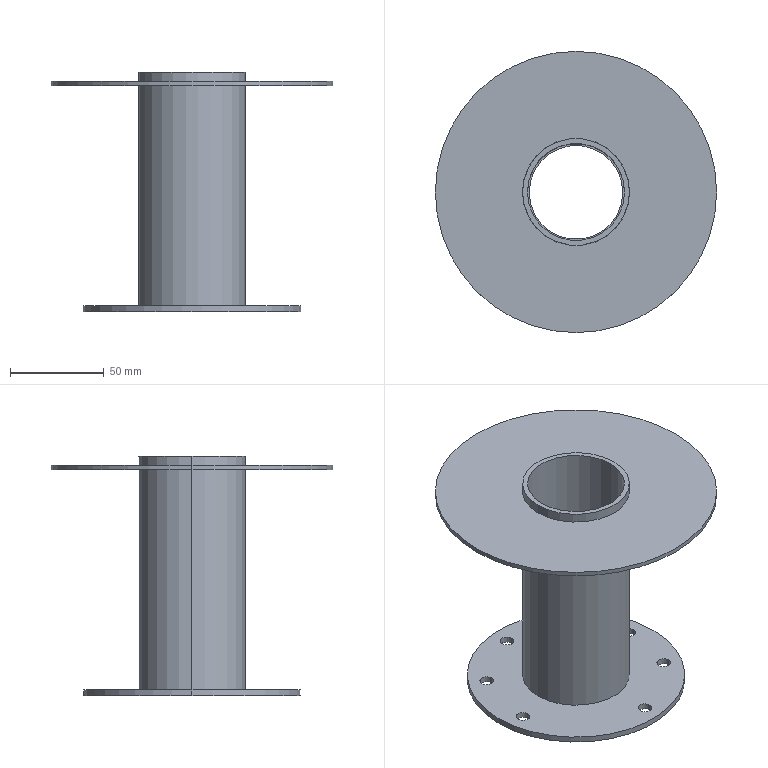Part | SolidWorks | features BaseBody 5 | 3 solids | 30 faces | box 150 x 150 x 127.9 mm | volume 116898 mm3 | cylinder 24 | plane 6 | commonest cylinder face diameters 7.2 x12 50 x2 51.8 x2 57 x2 57.2 x2 116 x2
STEP:
#1=CARTESIAN_POINT('',(-38.144,24.146,84.393));
#2=VERTEX_POINT('',#1);
#3=CARTESIAN_POINT('',(19.056,24.146,84.393));
#4=VERTEX_POINT('',#3);
#5=CARTESIAN_POINT('',(-9.544,24.146,84.393));
#6=DIRECTION('',(0.,0.,1.));
#7=DIRECTION('',(1.,0.,0.));
#8=AXIS2_PLACEMENT_3D('',#5,#6,#7);
#9=CIRCLE('',#8,28.6);
#10=EDGE_CURVE('',#2,#4,#9,.T.);
#11=ORIENTED_EDGE('',*,*,#10,.F.);
#12=CARTESIAN_POINT('',(-38.144,24.146,86.693));
#13=VERTEX_POINT('',#12);
#14=CARTESIAN_POINT('',(-38.144,24.146,84.393));
#15=DIRECTION('',(0.,0.,1.));
#16=VECTOR('',#15,1000.);
#17=LINE('',#14,#16);
#18=EDGE_CURVE('',#2,#13,#17,.T.);
#19=ORIENTED_EDGE('',*,*,#18,.T.);
#20=CARTESIAN_POINT('',(19.056,24.146,86.693));
#21=VERTEX_POINT('',#20);
#22=CARTESIAN_POINT('',(-9.544,24.146,86.693));
#23=DIRECTION('',(0.,0.,1.));
#24=DIRECTION('',(1.,0.,0.));
#25=AXIS2_PLACEMENT_3D('',#22,#23,#24);
#26=CIRCLE('',#25,28.6);
#27=EDGE_CURVE('',#13,#21,#26,.T.);
#28=ORIENTED_EDGE('',*,*,#27,.T.);
#29=CARTESIAN_POINT('',(19.056,24.146,84.393));
#30=DIRECTION('',(0.,0.,1.));
#31=VECTOR('',#30,1000.);
#32=LINE('',#29,#31);
#33=EDGE_CURVE('',#4,#21,#32,.T.);
#34=ORIENTED_EDGE('',*,*,#33,.F.);
#35=EDGE_LOOP('',(#11,#19,#28,#34));
#36=FACE_OUTER_BOUND('',#35,.T.);
#37=CARTESIAN_POINT('',(-9.544,24.146,84.393));
#38=DIRECTION('',(0.,0.,1.));
#39=DIRECTION('',(1.,0.,0.));
#40=AXIS2_PLACEMENT_3D('',#37,#38,#39);
#41=CYLINDRICAL_SURFACE('',#40,28.6);
#42=ADVANCED_FACE('',(#36),#41,.F.);
#43=CARTESIAN_POINT('',(65.456,24.146,84.393));
#44=VERTEX_POINT('',#43);
#45=CARTESIAN_POINT('',(-84.544,24.146,84.393));
#46=VERTEX_POINT('',#45);
#47=CARTESIAN_POINT('',(-9.544,24.146,84.393));
#48=DIRECTION('',(0.,0.,1.));
#49=DIRECTION('',(1.,0.,0.));
#50=AXIS2_PLACEMENT_3D('',#47,#48,#49);
#51=CIRCLE('',#50,75.);
#52=EDGE_CURVE('',#44,#46,#51,.T.);
#53=ORIENTED_EDGE('',*,*,#52,.T.);
#54=CARTESIAN_POINT('',(-84.544,24.146,86.693));
#55=VERTEX_POINT('',#54);
#56=CARTESIAN_POINT('',(-84.544,24.146,84.393));
#57=DIRECTION('',(0.,0.,1.));
#58=VECTOR('',#57,1000.);
#59=LINE('',#56,#58);
#60=EDGE_CURVE('',#46,#55,#59,.T.);
#61=ORIENTED_EDGE('',*,*,#60,.T.);
#62=CARTESIAN_POINT('',(65.456,24.146,86.693));
#63=VERTEX_POINT('',#62);
#64=CARTESIAN_POINT('',(-9.544,24.146,86.693));
#65=DIRECTION('',(0.,0.,1.));
#66=DIRECTION('',(1.,0.,0.));
#67=AXIS2_PLACEMENT_3D('',#64,#65,#66);
#68=CIRCLE('',#67,75.);
#69=EDGE_CURVE('',#63,#55,#68,.T.);
#70=ORIENTED_EDGE('',*,*,#69,.F.);
#71=CARTESIAN_POINT('',(65.456,24.146,84.393));
#72=DIRECTION('',(0.,0.,1.));
#73=VECTOR('',#72,1000.);
#74=LINE('',#71,#73);
#75=EDGE_CURVE('',#44,#63,#74,.T.);
#76=ORIENTED_EDGE('',*,*,#75,.F.);
#77=EDGE_LOOP('',(#53,#61,#70,#76));
#78=FACE_OUTER_BOUND('',#77,.T.);
#79=CARTESIAN_POINT('',(-9.544,24.146,84.393));
#80=DIRECTION('',(0.,0.,1.));
#81=DIRECTION('',(1.,0.,0.));
#82=AXIS2_PLACEMENT_3D('',#79,#80,#81);
#83=CYLINDRICAL_SURFACE('',#82,75.);
#84=ADVANCED_FACE('',(#78),#83,.T.);
#85=ORIENTED_EDGE('',*,*,#60,.F.);
#86=CARTESIAN_POINT('',(-9.544,24.146,84.393));
#87=DIRECTION('',(0.,0.,1.));
#88=DIRECTION('',(1.,0.,0.));
#89=AXIS2_PLACEMENT_3D('',#86,#87,#88);
#90=CIRCLE('',#89,75.);
#91=EDGE_CURVE('',#46,#44,#90,.T.);
#92=ORIENTED_EDGE('',*,*,#91,.T.);
#93=ORIENTED_EDGE('',*,*,#75,.T.);
#94=CARTESIAN_POINT('',(-9.544,24.146,86.693));
#95=DIRECTION('',(0.,0.,1.));
#96=DIRECTION('',(1.,0.,0.));
#97=AXIS2_PLACEMENT_3D('',#94,#95,#96);
#98=CIRCLE('',#97,75.);
#99=EDGE_CURVE('',#55,#63,#98,.T.);
#100=ORIENTED_EDGE('',*,*,#99,.F.);
#101=EDGE_LOOP('',(#85,#92,#93,#100));
#102=FACE_OUTER_BOUND('',#101,.T.);
#103=CARTESIAN_POINT('',(-9.544,24.146,84.393));
#104=DIRECTION('',(0.,0.,1.));
#105=DIRECTION('',(1.,0.,0.));
#106=AXIS2_PLACEMENT_3D('',#103,#104,#105);
#107=CYLINDRICAL_SURFACE('',#106,75.);
#108=ADVANCED_FACE('',(#102),#107,.T.);
#109=CARTESIAN_POINT('',(-9.544,24.146,84.393));
#110=DIRECTION('',(0.,0.,1.));
#111=DIRECTION('',(1.,0.,0.));
#112=AXIS2_PLACEMENT_3D('',#109,#110,#111);
#113=CIRCLE('',#112,28.6);
#114=EDGE_CURVE('',#4,#2,#113,.T.);
#115=ORIENTED_EDGE('',*,*,#114,.T.);
#116=ORIENTED_EDGE('',*,*,#10,.T.);
#117=EDGE_LOOP('',(#115,#116));
#118=FACE_BOUND('',#117,.T.);
#119=ORIENTED_EDGE('',*,*,#52,.F.);
#120=ORIENTED_EDGE('',*,*,#91,.F.);
#121=EDGE_LOOP('',(#119,#120));
#122=FACE_OUTER_BOUND('',#121,.T.);
#123=CARTESIAN_POINT('',(-9.544,24.146,84.393));
#124=DIRECTION('',(0.,0.,1.));
#125=DIRECTION('',(1.,0.,0.));
#126=AXIS2_PLACEMENT_3D('',#123,#124,#125);
#127=PLANE('',#126);
#128=ADVANCED_FACE('',(#118,#122),#127,.F.);
#129=CARTESIAN_POINT('',(-9.544,24.146,86.693));
#130=DIRECTION('',(0.,0.,1.));
#131=DIRECTION('',(1.,0.,0.));
#132=AXIS2_PLACEMENT_3D('',#129,#130,#131);
#133=CIRCLE('',#132,28.6);
#134=EDGE_CURVE('',#21,#13,#133,.T.);
#135=ORIENTED_EDGE('',*,*,#134,.F.);
#136=ORIENTED_EDGE('',*,*,#27,.F.);
#137=EDGE_LOOP('',(#135,#136));
#138=FACE_BOUND('',#137,.T.);
#139=ORIENTED_EDGE('',*,*,#69,.T.);
#140=ORIENTED_EDGE('',*,*,#99,.T.);
#141=EDGE_LOOP('',(#139,#140));
#142=FACE_OUTER_BOUND('',#141,.T.);
#143=CARTESIAN_POINT('',(-9.544,24.146,86.693));
#144=DIRECTION('',(0.,0.,1.));
#145=DIRECTION('',(1.,0.,0.));
#146=AXIS2_PLACEMENT_3D('',#143,#144,#145);
#147=PLANE('',#146);
#148=ADVANCED_FACE('',(#138,#142),#147,.T.);
#149=ORIENTED_EDGE('',*,*,#18,.F.);
#150=ORIENTED_EDGE('',*,*,#114,.F.);
#151=ORIENTED_EDGE('',*,*,#33,.T.);
#152=ORIENTED_EDGE('',*,*,#134,.T.);
#153=EDGE_LOOP('',(#149,#150,#151,#152));
#154=FACE_OUTER_BOUND('',#153,.T.);
#155=CARTESIAN_POINT('',(-9.544,24.146,84.393));
#156=DIRECTION('',(0.,0.,1.));
#157=DIRECTION('',(1.,0.,0.));
#158=AXIS2_PLACEMENT_3D('',#155,#156,#157);
#159=CYLINDRICAL_SURFACE('',#158,28.6);
#160=ADVANCED_FACE('',(#154),#159,.F.);
#161=CLOSED_SHELL('',(#42,#84,#108,#128,#148,#160));
#162=MANIFOLD_SOLID_BREP('',#161);
#163=CARTESIAN_POINT('',(-35.444,24.146,91.693));
#164=VERTEX_POINT('',#163);
#165=CARTESIAN_POINT('',(16.356,24.146,91.693));
#166=VERTEX_POINT('',#165);
#167=CARTESIAN_POINT('',(-9.544,24.146,91.693));
#168=DIRECTION('',(0.,0.,1.));
#169=DIRECTION('',(1.,0.,0.));
#170=AXIS2_PLACEMENT_3D('',#167,#168,#169);
#171=CIRCLE('',#170,25.9);
#172=EDGE_CURVE('',#164,#166,#171,.T.);
#173=ORIENTED_EDGE('',*,*,#172,.T.);
#174=CARTESIAN_POINT('',(16.356,24.146,-33.007));
#175=VERTEX_POINT('',#174);
#176=CARTESIAN_POINT('',(16.356,24.146,91.693));
#177=DIRECTION('',(0.,0.,-1.));
#178=VECTOR('',#177,1000.);
#179=LINE('',#176,#178);
#180=EDGE_CURVE('',#166,#175,#179,.T.);
#181=ORIENTED_EDGE('',*,*,#180,.T.);
#182=CARTESIAN_POINT('',(-35.444,24.146,-33.007));
#183=VERTEX_POINT('',#182);
#184=CARTESIAN_POINT('',(-9.544,24.146,-33.007));
#185=DIRECTION('',(0.,0.,1.));
#186=DIRECTION('',(1.,0.,0.));
#187=AXIS2_PLACEMENT_3D('',#184,#185,#186);
#188=CIRCLE('',#187,25.9);
#189=EDGE_CURVE('',#183,#175,#188,.T.);
#190=ORIENTED_EDGE('',*,*,#189,.F.);
#191=CARTESIAN_POINT('',(-35.444,24.146,91.693));
#192=DIRECTION('',(0.,0.,-1.));
#193=VECTOR('',#192,1000.);
#194=LINE('',#191,#193);
#195=EDGE_CURVE('',#164,#183,#194,.T.);
#196=ORIENTED_EDGE('',*,*,#195,.F.);
#197=EDGE_LOOP('',(#173,#181,#190,#196));
#198=FACE_OUTER_BOUND('',#197,.T.);
#199=CARTESIAN_POINT('',(-9.544,24.146,91.693));
#200=DIRECTION('',(0.,0.,-1.));
#201=DIRECTION('',(-1.,0.,0.));
#202=AXIS2_PLACEMENT_3D('',#199,#200,#201);
#203=CYLINDRICAL_SURFACE('',#202,25.9);
#204=ADVANCED_FACE('',(#198),#203,.F.);
#205=CARTESIAN_POINT('',(18.956,24.146,91.693));
#206=VERTEX_POINT('',#205);
#207=CARTESIAN_POINT('',(-38.044,24.146,91.693));
#208=VERTEX_POINT('',#207);
#209=CARTESIAN_POINT('',(-9.544,24.146,91.693));
#210=DIRECTION('',(0.,0.,1.));
#211=DIRECTION('',(1.,0.,0.));
#212=AXIS2_PLACEMENT_3D('',#209,#210,#211);
#213=CIRCLE('',#212,28.5);
#214=EDGE_CURVE('',#206,#208,#213,.T.);
#215=ORIENTED_EDGE('',*,*,#214,.F.);
#216=CARTESIAN_POINT('',(18.956,24.146,-33.007));
#217=VERTEX_POINT('',#216);
#218=CARTESIAN_POINT('',(18.956,24.146,91.693));
#219=DIRECTION('',(0.,0.,-1.));
#220=VECTOR('',#219,1000.);
#221=LINE('',#218,#220);
#222=EDGE_CURVE('',#206,#217,#221,.T.);
#223=ORIENTED_EDGE('',*,*,#222,.T.);
#224=CARTESIAN_POINT('',(-38.044,24.146,-33.007));
#225=VERTEX_POINT('',#224);
#226=CARTESIAN_POINT('',(-9.544,24.146,-33.007));
#227=DIRECTION('',(0.,0.,1.));
#228=DIRECTION('',(1.,0.,0.));
#229=AXIS2_PLACEMENT_3D('',#226,#227,#228);
#230=CIRCLE('',#229,28.5);
#231=EDGE_CURVE('',#217,#225,#230,.T.);
#232=ORIENTED_EDGE('',*,*,#231,.T.);
#233=CARTESIAN_POINT('',(-38.044,24.146,91.693));
#234=DIRECTION('',(0.,0.,-1.));
#235=VECTOR('',#234,1000.);
#236=LINE('',#233,#235);
#237=EDGE_CURVE('',#208,#225,#236,.T.);
#238=ORIENTED_EDGE('',*,*,#237,.F.);
#239=EDGE_LOOP('',(#215,#223,#232,#238));
#240=FACE_OUTER_BOUND('',#239,.T.);
#241=CARTESIAN_POINT('',(-9.544,24.146,91.693));
#242=DIRECTION('',(0.,0.,-1.));
#243=DIRECTION('',(-1.,0.,0.));
#244=AXIS2_PLACEMENT_3D('',#241,#242,#243);
#245=CYLINDRICAL_SURFACE('',#244,28.5);
#246=ADVANCED_FACE('',(#240),#245,.T.);
#247=CARTESIAN_POINT('',(-9.544,24.146,91.693));
#248=DIRECTION('',(0.,0.,1.));
#249=DIRECTION('',(1.,0.,0.));
#250=AXIS2_PLACEMENT_3D('',#247,#248,#249);
#251=CIRCLE('',#250,28.5);
#252=EDGE_CURVE('',#208,#206,#251,.T.);
#253=ORIENTED_EDGE('',*,*,#252,.T.);
#254=ORIENTED_EDGE('',*,*,#214,.T.);
#255=EDGE_LOOP('',(#253,#254));
#256=FACE_OUTER_BOUND('',#255,.T.);
#257=ORIENTED_EDGE('',*,*,#172,.F.);
#258=CARTESIAN_POINT('',(-9.544,24.146,91.693));
#259=DIRECTION('',(0.,0.,1.));
#260=DIRECTION('',(1.,0.,0.));
#261=AXIS2_PLACEMENT_3D('',#258,#259,#260);
#262=CIRCLE('',#261,25.9);
#263=EDGE_CURVE('',#166,#164,#262,.T.);
#264=ORIENTED_EDGE('',*,*,#263,.F.);
#265=EDGE_LOOP('',(#257,#264));
#266=FACE_BOUND('',#265,.T.);
#267=CARTESIAN_POINT('',(-9.544,24.146,91.693));
#268=DIRECTION('',(0.,0.,1.));
#269=DIRECTION('',(1.,0.,0.));
#270=AXIS2_PLACEMENT_3D('',#267,#268,#269);
#271=PLANE('',#270);
#272=ADVANCED_FACE('',(#256,#266),#271,.T.);
#273=CARTESIAN_POINT('',(-9.544,24.146,-33.007));
#274=DIRECTION('',(0.,0.,1.));
#275=DIRECTION('',(1.,0.,0.));
#276=AXIS2_PLACEMENT_3D('',#273,#274,#275);
#277=CIRCLE('',#276,28.5);
#278=EDGE_CURVE('',#225,#217,#277,.T.);
#279=ORIENTED_EDGE('',*,*,#278,.F.);
#280=ORIENTED_EDGE('',*,*,#231,.F.);
#281=EDGE_LOOP('',(#279,#280));
#282=FACE_OUTER_BOUND('',#281,.T.);
#283=ORIENTED_EDGE('',*,*,#189,.T.);
#284=CARTESIAN_POINT('',(-9.544,24.146,-33.007));
#285=DIRECTION('',(0.,0.,1.));
#286=DIRECTION('',(1.,0.,0.));
#287=AXIS2_PLACEMENT_3D('',#284,#285,#286);
#288=CIRCLE('',#287,25.9);
#289=EDGE_CURVE('',#175,#183,#288,.T.);
#290=ORIENTED_EDGE('',*,*,#289,.T.);
#291=EDGE_LOOP('',(#283,#290));
#292=FACE_BOUND('',#291,.T.);
#293=CARTESIAN_POINT('',(-9.544,24.146,-33.007));
#294=DIRECTION('',(0.,0.,1.));
#295=DIRECTION('',(1.,0.,0.));
#296=AXIS2_PLACEMENT_3D('',#293,#294,#295);
#297=PLANE('',#296);
#298=ADVANCED_FACE('',(#282,#292),#297,.F.);
#299=ORIENTED_EDGE('',*,*,#222,.F.);
#300=ORIENTED_EDGE('',*,*,#252,.F.);
#301=ORIENTED_EDGE('',*,*,#237,.T.);
#302=ORIENTED_EDGE('',*,*,#278,.T.);
#303=EDGE_LOOP('',(#299,#300,#301,#302));
#304=FACE_OUTER_BOUND('',#303,.T.);
#305=CARTESIAN_POINT('',(-9.544,24.146,91.693));
#306=DIRECTION('',(0.,0.,-1.));
#307=DIRECTION('',(-1.,0.,0.));
#308=AXIS2_PLACEMENT_3D('',#305,#306,#307);
#309=CYLINDRICAL_SURFACE('',#308,28.5);
#310=ADVANCED_FACE('',(#304),#309,.T.);
#311=ORIENTED_EDGE('',*,*,#180,.F.);
#312=ORIENTED_EDGE('',*,*,#263,.T.);
#313=ORIENTED_EDGE('',*,*,#195,.T.);
#314=ORIENTED_EDGE('',*,*,#289,.F.);
#315=EDGE_LOOP('',(#311,#312,#313,#314));
#316=FACE_OUTER_BOUND('',#315,.T.);
#317=CARTESIAN_POINT('',(-9.544,24.146,91.693));
#318=DIRECTION('',(0.,0.,-1.));
#319=DIRECTION('',(-1.,0.,0.));
#320=AXIS2_PLACEMENT_3D('',#317,#318,#319);
#321=CYLINDRICAL_SURFACE('',#320,25.9);
#322=ADVANCED_FACE('',(#316),#321,.F.);
#323=CLOSED_SHELL('',(#204,#246,#272,#298,#310,#322));
#324=MANIFOLD_SOLID_BREP('',#323);
#325=CARTESIAN_POINT('',(-17.328,71.964,-33.007));
#326=VERTEX_POINT('',#325);
#327=CARTESIAN_POINT('',(-10.128,71.964,-33.007));
#328=VERTEX_POINT('',#327);
#329=CARTESIAN_POINT('',(-13.728,71.964,-33.007));
#330=DIRECTION('',(0.,0.,-1.));
#331=DIRECTION('',(1.,0.,0.));
#332=AXIS2_PLACEMENT_3D('',#329,#330,#331);
#333=CIRCLE('',#332,3.6);
#334=EDGE_CURVE('',#326,#328,#333,.T.);
#335=ORIENTED_EDGE('',*,*,#334,.F.);
#336=CARTESIAN_POINT('',(-17.328,71.964,-36.207));
#337=VERTEX_POINT('',#336);
#338=CARTESIAN_POINT('',(-17.328,71.964,-33.007));
#339=DIRECTION('',(0.,0.,-1.));
#340=VECTOR('',#339,1000.);
#341=LINE('',#338,#340);
#342=EDGE_CURVE('',#326,#337,#341,.T.);
#343=ORIENTED_EDGE('',*,*,#342,.T.);
#344=CARTESIAN_POINT('',(-10.128,71.964,-36.207));
#345=VERTEX_POINT('',#344);
#346=CARTESIAN_POINT('',(-13.728,71.964,-36.207));
#347=DIRECTION('',(0.,0.,-1.));
#348=DIRECTION('',(1.,0.,0.));
#349=AXIS2_PLACEMENT_3D('',#346,#347,#348);
#350=CIRCLE('',#349,3.6);
#351=EDGE_CURVE('',#337,#345,#350,.T.);
#352=ORIENTED_EDGE('',*,*,#351,.T.);
#353=CARTESIAN_POINT('',(-10.128,71.964,-33.007));
#354=DIRECTION('',(0.,0.,-1.));
#355=VECTOR('',#354,1000.);
#356=LINE('',#353,#355);
#357=EDGE_CURVE('',#328,#345,#356,.T.);
#358=ORIENTED_EDGE('',*,*,#357,.F.);
#359=EDGE_LOOP('',(#335,#343,#352,#358));
#360=FACE_OUTER_BOUND('',#359,.T.);
#361=CARTESIAN_POINT('',(-13.728,71.964,-33.007));
#362=DIRECTION('',(0.,0.,-1.));
#363=DIRECTION('',(1.,0.,0.));
#364=AXIS2_PLACEMENT_3D('',#361,#362,#363);
#365=CYLINDRICAL_SURFACE('',#364,3.6);
#366=ADVANCED_FACE('',(#360),#365,.F.);
#367=CARTESIAN_POINT('',(-50.969,53.698,-33.007));
#368=VERTEX_POINT('',#367);
#369=CARTESIAN_POINT('',(-43.769,53.698,-33.007));
#370=VERTEX_POINT('',#369);
#371=CARTESIAN_POINT('',(-47.369,53.698,-33.007));
#372=DIRECTION('',(0.,0.,-1.));
#373=DIRECTION('',(1.,0.,0.));
#374=AXIS2_PLACEMENT_3D('',#371,#372,#373);
#375=CIRCLE('',#374,3.6);
#376=EDGE_CURVE('',#368,#370,#375,.T.);
#377=ORIENTED_EDGE('',*,*,#376,.F.);
#378=CARTESIAN_POINT('',(-50.969,53.698,-36.207));
#379=VERTEX_POINT('',#378);
#380=CARTESIAN_POINT('',(-50.969,53.698,-33.007));
#381=DIRECTION('',(0.,0.,-1.));
#382=VECTOR('',#381,1000.);
#383=LINE('',#380,#382);
#384=EDGE_CURVE('',#368,#379,#383,.T.);
#385=ORIENTED_EDGE('',*,*,#384,.T.);
#386=CARTESIAN_POINT('',(-43.769,53.698,-36.207));
#387=VERTEX_POINT('',#386);
#388=CARTESIAN_POINT('',(-47.369,53.698,-36.207));
#389=DIRECTION('',(0.,0.,-1.));
#390=DIRECTION('',(1.,0.,0.));
#391=AXIS2_PLACEMENT_3D('',#388,#389,#390);
#392=CIRCLE('',#391,3.6);
#393=EDGE_CURVE('',#379,#387,#392,.T.);
#394=ORIENTED_EDGE('',*,*,#393,.T.);
#395=CARTESIAN_POINT('',(-43.769,53.698,-33.007));
#396=DIRECTION('',(0.,0.,-1.));
#397=VECTOR('',#396,1000.);
#398=LINE('',#395,#397);
#399=EDGE_CURVE('',#370,#387,#398,.T.);
#400=ORIENTED_EDGE('',*,*,#399,.F.);
#401=EDGE_LOOP('',(#377,#385,#394,#400));
#402=FACE_OUTER_BOUND('',#401,.T.);
#403=CARTESIAN_POINT('',(-47.369,53.698,-33.007));
#404=DIRECTION('',(0.,0.,-1.));
#405=DIRECTION('',(1.,0.,0.));
#406=AXIS2_PLACEMENT_3D('',#403,#404,#405);
#407=CYLINDRICAL_SURFACE('',#406,3.6);
#408=ADVANCED_FACE('',(#402),#407,.F.);
#409=CARTESIAN_POINT('',(34.265,31.655,-33.007));
#410=VERTEX_POINT('',#409);
#411=CARTESIAN_POINT('',(41.465,31.655,-33.007));
#412=VERTEX_POINT('',#411);
#413=CARTESIAN_POINT('',(37.865,31.655,-33.007));
#414=DIRECTION('',(0.,0.,-1.));
#415=DIRECTION('',(1.,0.,0.));
#416=AXIS2_PLACEMENT_3D('',#413,#414,#415);
#417=CIRCLE('',#416,3.6);
#418=EDGE_CURVE('',#410,#412,#417,.T.);
#419=ORIENTED_EDGE('',*,*,#418,.F.);
#420=CARTESIAN_POINT('',(34.265,31.655,-36.207));
#421=VERTEX_POINT('',#420);
#422=CARTESIAN_POINT('',(34.265,31.655,-33.007));
#423=DIRECTION('',(0.,0.,-1.));
#424=VECTOR('',#423,1000.);
#425=LINE('',#422,#424);
#426=EDGE_CURVE('',#410,#421,#425,.T.);
#427=ORIENTED_EDGE('',*,*,#426,.T.);
#428=CARTESIAN_POINT('',(41.465,31.655,-36.207));
#429=VERTEX_POINT('',#428);
#430=CARTESIAN_POINT('',(37.865,31.655,-36.207));
#431=DIRECTION('',(0.,0.,-1.));
#432=DIRECTION('',(1.,0.,0.));
#433=AXIS2_PLACEMENT_3D('',#430,#431,#432);
#434=CIRCLE('',#433,3.6);
#435=EDGE_CURVE('',#421,#429,#434,.T.);
#436=ORIENTED_EDGE('',*,*,#435,.T.);
#437=CARTESIAN_POINT('',(41.465,31.655,-33.007));
#438=DIRECTION('',(0.,0.,-1.));
#439=VECTOR('',#438,1000.);
#440=LINE('',#437,#439);
#441=EDGE_CURVE('',#412,#429,#440,.T.);
#442=ORIENTED_EDGE('',*,*,#441,.F.);
#443=EDGE_LOOP('',(#419,#427,#436,#442));
#444=FACE_OUTER_BOUND('',#443,.T.);
#445=CARTESIAN_POINT('',(37.865,31.655,-33.007));
#446=DIRECTION('',(0.,0.,-1.));
#447=DIRECTION('',(1.,0.,0.));
#448=AXIS2_PLACEMENT_3D('',#445,#446,#447);
#449=CYLINDRICAL_SURFACE('',#448,3.6);
#450=ADVANCED_FACE('',(#444),#449,.F.);
#451=CARTESIAN_POINT('',(27.562,-1.29,-33.007));
#452=VERTEX_POINT('',#451);
#453=CARTESIAN_POINT('',(34.762,-1.29,-33.007));
#454=VERTEX_POINT('',#453);
#455=CARTESIAN_POINT('',(31.162,-1.29,-33.007));
#456=DIRECTION('',(0.,0.,-1.));
#457=DIRECTION('',(1.,0.,0.));
#458=AXIS2_PLACEMENT_3D('',#455,#456,#457);
#459=CIRCLE('',#458,3.6);
#460=EDGE_CURVE('',#452,#454,#459,.T.);
#461=ORIENTED_EDGE('',*,*,#460,.F.);
#462=CARTESIAN_POINT('',(27.562,-1.29,-36.207));
#463=VERTEX_POINT('',#462);
#464=CARTESIAN_POINT('',(27.562,-1.29,-33.007));
#465=DIRECTION('',(0.,0.,-1.));
#466=VECTOR('',#465,1000.);
#467=LINE('',#464,#466);
#468=EDGE_CURVE('',#452,#463,#467,.T.);
#469=ORIENTED_EDGE('',*,*,#468,.T.);
#470=CARTESIAN_POINT('',(34.762,-1.29,-36.207));
#471=VERTEX_POINT('',#470);
#472=CARTESIAN_POINT('',(31.162,-1.29,-36.207));
#473=DIRECTION('',(0.,0.,-1.));
#474=DIRECTION('',(1.,0.,0.));
#475=AXIS2_PLACEMENT_3D('',#472,#473,#474);
#476=CIRCLE('',#475,3.6);
#477=EDGE_CURVE('',#463,#471,#476,.T.);
#478=ORIENTED_EDGE('',*,*,#477,.T.);
#479=CARTESIAN_POINT('',(34.762,-1.29,-33.007));
#480=DIRECTION('',(0.,0.,-1.));
#481=VECTOR('',#480,1000.);
#482=LINE('',#479,#481);
#483=EDGE_CURVE('',#454,#471,#482,.T.);
#484=ORIENTED_EDGE('',*,*,#483,.F.);
#485=EDGE_LOOP('',(#461,#469,#478,#484));
#486=FACE_OUTER_BOUND('',#485,.T.);
#487=CARTESIAN_POINT('',(31.162,-1.29,-33.007));
#488=DIRECTION('',(0.,0.,-1.));
#489=DIRECTION('',(1.,0.,0.));
#490=AXIS2_PLACEMENT_3D('',#487,#488,#489);
#491=CYLINDRICAL_SURFACE('',#490,3.6);
#492=ADVANCED_FACE('',(#486),#491,.F.);
#493=CARTESIAN_POINT('',(-8.961,-23.671,-33.007));
#494=VERTEX_POINT('',#493);
#495=CARTESIAN_POINT('',(-1.761,-23.671,-33.007));
#496=VERTEX_POINT('',#495);
#497=CARTESIAN_POINT('',(-5.361,-23.671,-33.007));
#498=DIRECTION('',(0.,0.,-1.));
#499=DIRECTION('',(1.,0.,0.));
#500=AXIS2_PLACEMENT_3D('',#497,#498,#499);
#501=CIRCLE('',#500,3.6);
#502=EDGE_CURVE('',#494,#496,#501,.T.);
#503=ORIENTED_EDGE('',*,*,#502,.F.);
#504=CARTESIAN_POINT('',(-8.961,-23.671,-36.207));
#505=VERTEX_POINT('',#504);
#506=CARTESIAN_POINT('',(-8.961,-23.671,-33.007));
#507=DIRECTION('',(0.,0.,-1.));
#508=VECTOR('',#507,1000.);
#509=LINE('',#506,#508);
#510=EDGE_CURVE('',#494,#505,#509,.T.);
#511=ORIENTED_EDGE('',*,*,#510,.T.);
#512=CARTESIAN_POINT('',(-1.761,-23.671,-36.207));
#513=VERTEX_POINT('',#512);
#514=CARTESIAN_POINT('',(-5.361,-23.671,-36.207));
#515=DIRECTION('',(0.,0.,-1.));
#516=DIRECTION('',(1.,0.,0.));
#517=AXIS2_PLACEMENT_3D('',#514,#515,#516);
#518=CIRCLE('',#517,3.6);
#519=EDGE_CURVE('',#505,#513,#518,.T.);
#520=ORIENTED_EDGE('',*,*,#519,.T.);
#521=CARTESIAN_POINT('',(-1.761,-23.671,-33.007));
#522=DIRECTION('',(0.,0.,-1.));
#523=VECTOR('',#522,1000.);
#524=LINE('',#521,#523);
#525=EDGE_CURVE('',#496,#513,#524,.T.);
#526=ORIENTED_EDGE('',*,*,#525,.F.);
#527=EDGE_LOOP('',(#503,#511,#520,#526));
#528=FACE_OUTER_BOUND('',#527,.T.);
#529=CARTESIAN_POINT('',(-5.361,-23.671,-33.007));
#530=DIRECTION('',(0.,0.,-1.));
#531=DIRECTION('',(1.,0.,0.));
#532=AXIS2_PLACEMENT_3D('',#529,#530,#531);
#533=CYLINDRICAL_SURFACE('',#532,3.6);
#534=ADVANCED_FACE('',(#528),#533,.F.);
#535=CARTESIAN_POINT('',(-60.554,16.637,-33.007));
#536=VERTEX_POINT('',#535);
#537=CARTESIAN_POINT('',(-53.354,16.637,-33.007));
#538=VERTEX_POINT('',#537);
#539=CARTESIAN_POINT('',(-56.954,16.637,-33.007));
#540=DIRECTION('',(0.,0.,-1.));
#541=DIRECTION('',(1.,0.,0.));
#542=AXIS2_PLACEMENT_3D('',#539,#540,#541);
#543=CIRCLE('',#542,3.6);
#544=EDGE_CURVE('',#536,#538,#543,.T.);
#545=ORIENTED_EDGE('',*,*,#544,.F.);
#546=CARTESIAN_POINT('',(-60.554,16.637,-36.207));
#547=VERTEX_POINT('',#546);
#548=CARTESIAN_POINT('',(-60.554,16.637,-33.007));
#549=DIRECTION('',(0.,0.,-1.));
#550=VECTOR('',#549,1000.);
#551=LINE('',#548,#550);
#552=EDGE_CURVE('',#536,#547,#551,.T.);
#553=ORIENTED_EDGE('',*,*,#552,.T.);
#554=CARTESIAN_POINT('',(-53.354,16.637,-36.207));
#555=VERTEX_POINT('',#554);
#556=CARTESIAN_POINT('',(-56.954,16.637,-36.207));
#557=DIRECTION('',(0.,0.,-1.));
#558=DIRECTION('',(1.,0.,0.));
#559=AXIS2_PLACEMENT_3D('',#556,#557,#558);
#560=CIRCLE('',#559,3.6);
#561=EDGE_CURVE('',#547,#555,#560,.T.);
#562=ORIENTED_EDGE('',*,*,#561,.T.);
#563=CARTESIAN_POINT('',(-53.354,16.637,-33.007));
#564=DIRECTION('',(0.,0.,-1.));
#565=VECTOR('',#564,1000.);
#566=LINE('',#563,#565);
#567=EDGE_CURVE('',#538,#555,#566,.T.);
#568=ORIENTED_EDGE('',*,*,#567,.F.);
#569=EDGE_LOOP('',(#545,#553,#562,#568));
#570=FACE_OUTER_BOUND('',#569,.T.);
#571=CARTESIAN_POINT('',(-56.954,16.637,-33.007));
#572=DIRECTION('',(0.,0.,-1.));
#573=DIRECTION('',(1.,0.,0.));
#574=AXIS2_PLACEMENT_3D('',#571,#572,#573);
#575=CYLINDRICAL_SURFACE('',#574,3.6);
#576=ADVANCED_FACE('',(#570),#575,.F.);
#577=CARTESIAN_POINT('',(-34.544,24.146,-33.007));
#578=VERTEX_POINT('',#577);
#579=CARTESIAN_POINT('',(15.456,24.146,-33.007));
#580=VERTEX_POINT('',#579);
#581=CARTESIAN_POINT('',(-9.544,24.146,-33.007));
#582=DIRECTION('',(0.,0.,-1.));
#583=DIRECTION('',(1.,0.,0.));
#584=AXIS2_PLACEMENT_3D('',#581,#582,#583);
#585=CIRCLE('',#584,25.);
#586=EDGE_CURVE('',#578,#580,#585,.T.);
#587=ORIENTED_EDGE('',*,*,#586,.F.);
#588=CARTESIAN_POINT('',(-34.544,24.146,-36.207));
#589=VERTEX_POINT('',#588);
#590=CARTESIAN_POINT('',(-34.544,24.146,-33.007));
#591=DIRECTION('',(0.,0.,-1.));
#592=VECTOR('',#591,1000.);
#593=LINE('',#590,#592);
#594=EDGE_CURVE('',#578,#589,#593,.T.);
#595=ORIENTED_EDGE('',*,*,#594,.T.);
#596=CARTESIAN_POINT('',(15.456,24.146,-36.207));
#597=VERTEX_POINT('',#596);
#598=CARTESIAN_POINT('',(-9.544,24.146,-36.207));
#599=DIRECTION('',(0.,0.,-1.));
#600=DIRECTION('',(1.,0.,0.));
#601=AXIS2_PLACEMENT_3D('',#598,#599,#600);
#602=CIRCLE('',#601,25.);
#603=EDGE_CURVE('',#589,#597,#602,.T.);
#604=ORIENTED_EDGE('',*,*,#603,.T.);
#605=CARTESIAN_POINT('',(15.456,24.146,-33.007));
#606=DIRECTION('',(0.,0.,-1.));
#607=VECTOR('',#606,1000.);
#608=LINE('',#605,#607);
#609=EDGE_CURVE('',#580,#597,#608,.T.);
#610=ORIENTED_EDGE('',*,*,#609,.F.);
#611=EDGE_LOOP('',(#587,#595,#604,#610));
#612=FACE_OUTER_BOUND('',#611,.T.);
#613=CARTESIAN_POINT('',(-9.544,24.146,-33.007));
#614=DIRECTION('',(0.,0.,-1.));
#615=DIRECTION('',(1.,0.,0.));
#616=AXIS2_PLACEMENT_3D('',#613,#614,#615);
#617=CYLINDRICAL_SURFACE('',#616,25.);
#618=ADVANCED_FACE('',(#612),#617,.F.);
#619=CARTESIAN_POINT('',(48.456,24.146,-33.007));
#620=VERTEX_POINT('',#619);
#621=CARTESIAN_POINT('',(-67.544,24.146,-33.007));
#622=VERTEX_POINT('',#621);
#623=CARTESIAN_POINT('',(-9.544,24.146,-33.007));
#624=DIRECTION('',(0.,0.,-1.));
#625=DIRECTION('',(1.,0.,0.));
#626=AXIS2_PLACEMENT_3D('',#623,#624,#625);
#627=CIRCLE('',#626,58.);
#628=EDGE_CURVE('',#620,#622,#627,.T.);
#629=ORIENTED_EDGE('',*,*,#628,.T.);
#630=CARTESIAN_POINT('',(-67.544,24.146,-36.207));
#631=VERTEX_POINT('',#630);
#632=CARTESIAN_POINT('',(-67.544,24.146,-33.007));
#633=DIRECTION('',(0.,0.,-1.));
#634=VECTOR('',#633,1000.);
#635=LINE('',#632,#634);
#636=EDGE_CURVE('',#622,#631,#635,.T.);
#637=ORIENTED_EDGE('',*,*,#636,.T.);
#638=CARTESIAN_POINT('',(48.456,24.146,-36.207));
#639=VERTEX_POINT('',#638);
#640=CARTESIAN_POINT('',(-9.544,24.146,-36.207));
#641=DIRECTION('',(0.,0.,-1.));
#642=DIRECTION('',(1.,0.,0.));
#643=AXIS2_PLACEMENT_3D('',#640,#641,#642);
#644=CIRCLE('',#643,58.);
#645=EDGE_CURVE('',#639,#631,#644,.T.);
#646=ORIENTED_EDGE('',*,*,#645,.F.);
#647=CARTESIAN_POINT('',(48.456,24.146,-33.007));
#648=DIRECTION('',(0.,0.,-1.));
#649=VECTOR('',#648,1000.);
#650=LINE('',#647,#649);
#651=EDGE_CURVE('',#620,#639,#650,.T.);
#652=ORIENTED_EDGE('',*,*,#651,.F.);
#653=EDGE_LOOP('',(#629,#637,#646,#652));
#654=FACE_OUTER_BOUND('',#653,.T.);
#655=CARTESIAN_POINT('',(-9.544,24.146,-33.007));
#656=DIRECTION('',(0.,0.,-1.));
#657=DIRECTION('',(1.,0.,0.));
#658=AXIS2_PLACEMENT_3D('',#655,#656,#657);
#659=CYLINDRICAL_SURFACE('',#658,58.);
#660=ADVANCED_FACE('',(#654),#659,.T.);
#661=ORIENTED_EDGE('',*,*,#636,.F.);
#662=CARTESIAN_POINT('',(-9.544,24.146,-33.007));
#663=DIRECTION('',(0.,0.,-1.));
#664=DIRECTION('',(1.,0.,0.));
#665=AXIS2_PLACEMENT_3D('',#662,#663,#664);
#666=CIRCLE('',#665,58.);
#667=EDGE_CURVE('',#622,#620,#666,.T.);
#668=ORIENTED_EDGE('',*,*,#667,.T.);
#669=ORIENTED_EDGE('',*,*,#651,.T.);
#670=CARTESIAN_POINT('',(-9.544,24.146,-36.207));
#671=DIRECTION('',(0.,0.,-1.));
#672=DIRECTION('',(1.,0.,0.));
#673=AXIS2_PLACEMENT_3D('',#670,#671,#672);
#674=CIRCLE('',#673,58.);
#675=EDGE_CURVE('',#631,#639,#674,.T.);
#676=ORIENTED_EDGE('',*,*,#675,.F.);
#677=EDGE_LOOP('',(#661,#668,#669,#676));
#678=FACE_OUTER_BOUND('',#677,.T.);
#679=CARTESIAN_POINT('',(-9.544,24.146,-33.007));
#680=DIRECTION('',(0.,0.,-1.));
#681=DIRECTION('',(1.,0.,0.));
#682=AXIS2_PLACEMENT_3D('',#679,#680,#681);
#683=CYLINDRICAL_SURFACE('',#682,58.);
#684=ADVANCED_FACE('',(#678),#683,.T.);
#685=CARTESIAN_POINT('',(-13.728,71.964,-33.007));
#686=DIRECTION('',(0.,0.,-1.));
#687=DIRECTION('',(1.,0.,0.));
#688=AXIS2_PLACEMENT_3D('',#685,#686,#687);
#689=CIRCLE('',#688,3.6);
#690=EDGE_CURVE('',#328,#326,#689,.T.);
#691=ORIENTED_EDGE('',*,*,#690,.T.);
#692=ORIENTED_EDGE('',*,*,#334,.T.);
#693=EDGE_LOOP('',(#691,#692));
#694=FACE_BOUND('',#693,.T.);
#695=CARTESIAN_POINT('',(-47.369,53.698,-33.007));
#696=DIRECTION('',(0.,0.,-1.));
#697=DIRECTION('',(1.,0.,0.));
#698=AXIS2_PLACEMENT_3D('',#695,#696,#697);
#699=CIRCLE('',#698,3.6);
#700=EDGE_CURVE('',#370,#368,#699,.T.);
#701=ORIENTED_EDGE('',*,*,#700,.T.);
#702=ORIENTED_EDGE('',*,*,#376,.T.);
#703=EDGE_LOOP('',(#701,#702));
#704=FACE_BOUND('',#703,.T.);
#705=CARTESIAN_POINT('',(37.865,31.655,-33.007));
#706=DIRECTION('',(0.,0.,-1.));
#707=DIRECTION('',(1.,0.,0.));
#708=AXIS2_PLACEMENT_3D('',#705,#706,#707);
#709=CIRCLE('',#708,3.6);
#710=EDGE_CURVE('',#412,#410,#709,.T.);
#711=ORIENTED_EDGE('',*,*,#710,.T.);
#712=ORIENTED_EDGE('',*,*,#418,.T.);
#713=EDGE_LOOP('',(#711,#712));
#714=FACE_BOUND('',#713,.T.);
#715=CARTESIAN_POINT('',(31.162,-1.29,-33.007));
#716=DIRECTION('',(0.,0.,-1.));
#717=DIRECTION('',(1.,0.,0.));
#718=AXIS2_PLACEMENT_3D('',#715,#716,#717);
#719=CIRCLE('',#718,3.6);
#720=EDGE_CURVE('',#454,#452,#719,.T.);
#721=ORIENTED_EDGE('',*,*,#720,.T.);
#722=ORIENTED_EDGE('',*,*,#460,.T.);
#723=EDGE_LOOP('',(#721,#722));
#724=FACE_BOUND('',#723,.T.);
#725=CARTESIAN_POINT('',(-5.361,-23.671,-33.007));
#726=DIRECTION('',(0.,0.,-1.));
#727=DIRECTION('',(1.,0.,0.));
#728=AXIS2_PLACEMENT_3D('',#725,#726,#727);
#729=CIRCLE('',#728,3.6);
#730=EDGE_CURVE('',#496,#494,#729,.T.);
#731=ORIENTED_EDGE('',*,*,#730,.T.);
#732=ORIENTED_EDGE('',*,*,#502,.T.);
#733=EDGE_LOOP('',(#731,#732));
#734=FACE_BOUND('',#733,.T.);
#735=CARTESIAN_POINT('',(-56.954,16.637,-33.007));
#736=DIRECTION('',(0.,0.,-1.));
#737=DIRECTION('',(1.,0.,0.));
#738=AXIS2_PLACEMENT_3D('',#735,#736,#737);
#739=CIRCLE('',#738,3.6);
#740=EDGE_CURVE('',#538,#536,#739,.T.);
#741=ORIENTED_EDGE('',*,*,#740,.T.);
#742=ORIENTED_EDGE('',*,*,#544,.T.);
#743=EDGE_LOOP('',(#741,#742));
#744=FACE_BOUND('',#743,.T.);
#745=CARTESIAN_POINT('',(-9.544,24.146,-33.007));
#746=DIRECTION('',(0.,0.,-1.));
#747=DIRECTION('',(1.,0.,0.));
#748=AXIS2_PLACEMENT_3D('',#745,#746,#747);
#749=CIRCLE('',#748,25.);
#750=EDGE_CURVE('',#580,#578,#749,.T.);
#751=ORIENTED_EDGE('',*,*,#750,.T.);
#752=ORIENTED_EDGE('',*,*,#586,.T.);
#753=EDGE_LOOP('',(#751,#752));
#754=FACE_BOUND('',#753,.T.);
#755=ORIENTED_EDGE('',*,*,#628,.F.);
#756=ORIENTED_EDGE('',*,*,#667,.F.);
#757=EDGE_LOOP('',(#755,#756));
#758=FACE_OUTER_BOUND('',#757,.T.);
#759=CARTESIAN_POINT('',(-9.544,24.146,-33.007));
#760=DIRECTION('',(0.,0.,-1.));
#761=DIRECTION('',(1.,0.,0.));
#762=AXIS2_PLACEMENT_3D('',#759,#760,#761);
#763=PLANE('',#762);
#764=ADVANCED_FACE('',(#694,#704,#714,#724,#734,#744,#754,#758),#763,.F.);
#765=CARTESIAN_POINT('',(-13.728,71.964,-36.207));
#766=DIRECTION('',(0.,0.,-1.));
#767=DIRECTION('',(1.,0.,0.));
#768=AXIS2_PLACEMENT_3D('',#765,#766,#767);
#769=CIRCLE('',#768,3.6);
#770=EDGE_CURVE('',#345,#337,#769,.T.);
#771=ORIENTED_EDGE('',*,*,#770,.F.);
#772=ORIENTED_EDGE('',*,*,#351,.F.);
#773=EDGE_LOOP('',(#771,#772));
#774=FACE_BOUND('',#773,.T.);
#775=CARTESIAN_POINT('',(-47.369,53.698,-36.207));
#776=DIRECTION('',(0.,0.,-1.));
#777=DIRECTION('',(1.,0.,0.));
#778=AXIS2_PLACEMENT_3D('',#775,#776,#777);
#779=CIRCLE('',#778,3.6);
#780=EDGE_CURVE('',#387,#379,#779,.T.);
#781=ORIENTED_EDGE('',*,*,#780,.F.);
#782=ORIENTED_EDGE('',*,*,#393,.F.);
#783=EDGE_LOOP('',(#781,#782));
#784=FACE_BOUND('',#783,.T.);
#785=CARTESIAN_POINT('',(37.865,31.655,-36.207));
#786=DIRECTION('',(0.,0.,-1.));
#787=DIRECTION('',(1.,0.,0.));
#788=AXIS2_PLACEMENT_3D('',#785,#786,#787);
#789=CIRCLE('',#788,3.6);
#790=EDGE_CURVE('',#429,#421,#789,.T.);
#791=ORIENTED_EDGE('',*,*,#790,.F.);
#792=ORIENTED_EDGE('',*,*,#435,.F.);
#793=EDGE_LOOP('',(#791,#792));
#794=FACE_BOUND('',#793,.T.);
#795=CARTESIAN_POINT('',(31.162,-1.29,-36.207));
#796=DIRECTION('',(0.,0.,-1.));
#797=DIRECTION('',(1.,0.,0.));
#798=AXIS2_PLACEMENT_3D('',#795,#796,#797);
#799=CIRCLE('',#798,3.6);
#800=EDGE_CURVE('',#471,#463,#799,.T.);
#801=ORIENTED_EDGE('',*,*,#800,.F.);
#802=ORIENTED_EDGE('',*,*,#477,.F.);
#803=EDGE_LOOP('',(#801,#802));
#804=FACE_BOUND('',#803,.T.);
#805=CARTESIAN_POINT('',(-5.361,-23.671,-36.207));
#806=DIRECTION('',(0.,0.,-1.));
#807=DIRECTION('',(1.,0.,0.));
#808=AXIS2_PLACEMENT_3D('',#805,#806,#807);
#809=CIRCLE('',#808,3.6);
#810=EDGE_CURVE('',#513,#505,#809,.T.);
#811=ORIENTED_EDGE('',*,*,#810,.F.);
#812=ORIENTED_EDGE('',*,*,#519,.F.);
#813=EDGE_LOOP('',(#811,#812));
#814=FACE_BOUND('',#813,.T.);
#815=CARTESIAN_POINT('',(-56.954,16.637,-36.207));
#816=DIRECTION('',(0.,0.,-1.));
#817=DIRECTION('',(1.,0.,0.));
#818=AXIS2_PLACEMENT_3D('',#815,#816,#817);
#819=CIRCLE('',#818,3.6);
#820=EDGE_CURVE('',#555,#547,#819,.T.);
#821=ORIENTED_EDGE('',*,*,#820,.F.);
#822=ORIENTED_EDGE('',*,*,#561,.F.);
#823=EDGE_LOOP('',(#821,#822));
#824=FACE_BOUND('',#823,.T.);
#825=CARTESIAN_POINT('',(-9.544,24.146,-36.207));
#826=DIRECTION('',(0.,0.,-1.));
#827=DIRECTION('',(1.,0.,0.));
#828=AXIS2_PLACEMENT_3D('',#825,#826,#827);
#829=CIRCLE('',#828,25.);
#830=EDGE_CURVE('',#597,#589,#829,.T.);
#831=ORIENTED_EDGE('',*,*,#830,.F.);
#832=ORIENTED_EDGE('',*,*,#603,.F.);
#833=EDGE_LOOP('',(#831,#832));
#834=FACE_BOUND('',#833,.T.);
#835=ORIENTED_EDGE('',*,*,#645,.T.);
#836=ORIENTED_EDGE('',*,*,#675,.T.);
#837=EDGE_LOOP('',(#835,#836));
#838=FACE_OUTER_BOUND('',#837,.T.);
#839=CARTESIAN_POINT('',(-9.544,24.146,-36.207));
#840=DIRECTION('',(0.,0.,-1.));
#841=DIRECTION('',(1.,0.,0.));
#842=AXIS2_PLACEMENT_3D('',#839,#840,#841);
#843=PLANE('',#842);
#844=ADVANCED_FACE('',(#774,#784,#794,#804,#814,#824,#834,#838),#843,.T.);
#845=ORIENTED_EDGE('',*,*,#594,.F.);
#846=ORIENTED_EDGE('',*,*,#750,.F.);
#847=ORIENTED_EDGE('',*,*,#609,.T.);
#848=ORIENTED_EDGE('',*,*,#830,.T.);
#849=EDGE_LOOP('',(#845,#846,#847,#848));
#850=FACE_OUTER_BOUND('',#849,.T.);
#851=CARTESIAN_POINT('',(-9.544,24.146,-33.007));
#852=DIRECTION('',(0.,0.,-1.));
#853=DIRECTION('',(1.,0.,0.));
#854=AXIS2_PLACEMENT_3D('',#851,#852,#853);
#855=CYLINDRICAL_SURFACE('',#854,25.);
#856=ADVANCED_FACE('',(#850),#855,.F.);
#857=ORIENTED_EDGE('',*,*,#552,.F.);
#858=ORIENTED_EDGE('',*,*,#740,.F.);
#859=ORIENTED_EDGE('',*,*,#567,.T.);
#860=ORIENTED_EDGE('',*,*,#820,.T.);
#861=EDGE_LOOP('',(#857,#858,#859,#860));
#862=FACE_OUTER_BOUND('',#861,.T.);
#863=CARTESIAN_POINT('',(-56.954,16.637,-33.007));
#864=DIRECTION('',(0.,0.,-1.));
#865=DIRECTION('',(1.,0.,0.));
#866=AXIS2_PLACEMENT_3D('',#863,#864,#865);
#867=CYLINDRICAL_SURFACE('',#866,3.6);
#868=ADVANCED_FACE('',(#862),#867,.F.);
#869=ORIENTED_EDGE('',*,*,#510,.F.);
#870=ORIENTED_EDGE('',*,*,#730,.F.);
#871=ORIENTED_EDGE('',*,*,#525,.T.);
#872=ORIENTED_EDGE('',*,*,#810,.T.);
#873=EDGE_LOOP('',(#869,#870,#871,#872));
#874=FACE_OUTER_BOUND('',#873,.T.);
#875=CARTESIAN_POINT('',(-5.361,-23.671,-33.007));
#876=DIRECTION('',(0.,0.,-1.));
#877=DIRECTION('',(1.,0.,0.));
#878=AXIS2_PLACEMENT_3D('',#875,#876,#877);
#879=CYLINDRICAL_SURFACE('',#878,3.6);
#880=ADVANCED_FACE('',(#874),#879,.F.);
#881=ORIENTED_EDGE('',*,*,#468,.F.);
#882=ORIENTED_EDGE('',*,*,#720,.F.);
#883=ORIENTED_EDGE('',*,*,#483,.T.);
#884=ORIENTED_EDGE('',*,*,#800,.T.);
#885=EDGE_LOOP('',(#881,#882,#883,#884));
#886=FACE_OUTER_BOUND('',#885,.T.);
#887=CARTESIAN_POINT('',(31.162,-1.29,-33.007));
#888=DIRECTION('',(0.,0.,-1.));
#889=DIRECTION('',(1.,0.,0.));
#890=AXIS2_PLACEMENT_3D('',#887,#888,#889);
#891=CYLINDRICAL_SURFACE('',#890,3.6);
#892=ADVANCED_FACE('',(#886),#891,.F.);
#893=ORIENTED_EDGE('',*,*,#426,.F.);
#894=ORIENTED_EDGE('',*,*,#710,.F.);
#895=ORIENTED_EDGE('',*,*,#441,.T.);
#896=ORIENTED_EDGE('',*,*,#790,.T.);
#897=EDGE_LOOP('',(#893,#894,#895,#896));
#898=FACE_OUTER_BOUND('',#897,.T.);
#899=CARTESIAN_POINT('',(37.865,31.655,-33.007));
#900=DIRECTION('',(0.,0.,-1.));
#901=DIRECTION('',(1.,0.,0.));
#902=AXIS2_PLACEMENT_3D('',#899,#900,#901);
#903=CYLINDRICAL_SURFACE('',#902,3.6);
#904=ADVANCED_FACE('',(#898),#903,.F.);
#905=ORIENTED_EDGE('',*,*,#384,.F.);
#906=ORIENTED_EDGE('',*,*,#700,.F.);
#907=ORIENTED_EDGE('',*,*,#399,.T.);
#908=ORIENTED_EDGE('',*,*,#780,.T.);
#909=EDGE_LOOP('',(#905,#906,#907,#908));
#910=FACE_OUTER_BOUND('',#909,.T.);
#911=CARTESIAN_POINT('',(-47.369,53.698,-33.007));
#912=DIRECTION('',(0.,0.,-1.));
#913=DIRECTION('',(1.,0.,0.));
#914=AXIS2_PLACEMENT_3D('',#911,#912,#913);
#915=CYLINDRICAL_SURFACE('',#914,3.6);
#916=ADVANCED_FACE('',(#910),#915,.F.);
#917=ORIENTED_EDGE('',*,*,#342,.F.);
#918=ORIENTED_EDGE('',*,*,#690,.F.);
#919=ORIENTED_EDGE('',*,*,#357,.T.);
#920=ORIENTED_EDGE('',*,*,#770,.T.);
#921=EDGE_LOOP('',(#917,#918,#919,#920));
#922=FACE_OUTER_BOUND('',#921,.T.);
#923=CARTESIAN_POINT('',(-13.728,71.964,-33.007));
#924=DIRECTION('',(0.,0.,-1.));
#925=DIRECTION('',(1.,0.,0.));
#926=AXIS2_PLACEMENT_3D('',#923,#924,#925);
#927=CYLINDRICAL_SURFACE('',#926,3.6);
#928=ADVANCED_FACE('',(#922),#927,.F.);
#929=CLOSED_SHELL('',(#366,#408,#450,#492,#534,#576,#618,#660,#684,#764,#844,#856,#868,#880,#892,#904,#916,#928));
#930=MANIFOLD_SOLID_BREP('',#929);
#931=CARTESIAN_POINT('',(0.,0.,0.));
#932=DIRECTION('',(0.,0.,1.));
#933=DIRECTION('',(1.,0.,0.));
#934=AXIS2_PLACEMENT_3D('',#931,#932,#933);
#935=(LENGTH_UNIT()NAMED_UNIT(*)SI_UNIT(.MILLI.,.METRE.));
#936=UNCERTAINTY_MEASURE_WITH_UNIT(LENGTH_MEASURE(0.00001),#935,'','');
#937=(NAMED_UNIT(*)PLANE_ANGLE_UNIT()SI_UNIT($,.RADIAN.));
#938=(NAMED_UNIT(*)SI_UNIT($,.STERADIAN.)SOLID_ANGLE_UNIT());
#939=(GEOMETRIC_REPRESENTATION_CONTEXT(3)GLOBAL_UNCERTAINTY_ASSIGNED_CONTEXT((#936))GLOBAL_UNIT_ASSIGNED_CONTEXT((#935,#937,#938))REPRESENTATION_CONTEXT('',''));
#940=ADVANCED_BREP_SHAPE_REPRESENTATION('',(#162,#324,#930,#934),#939);